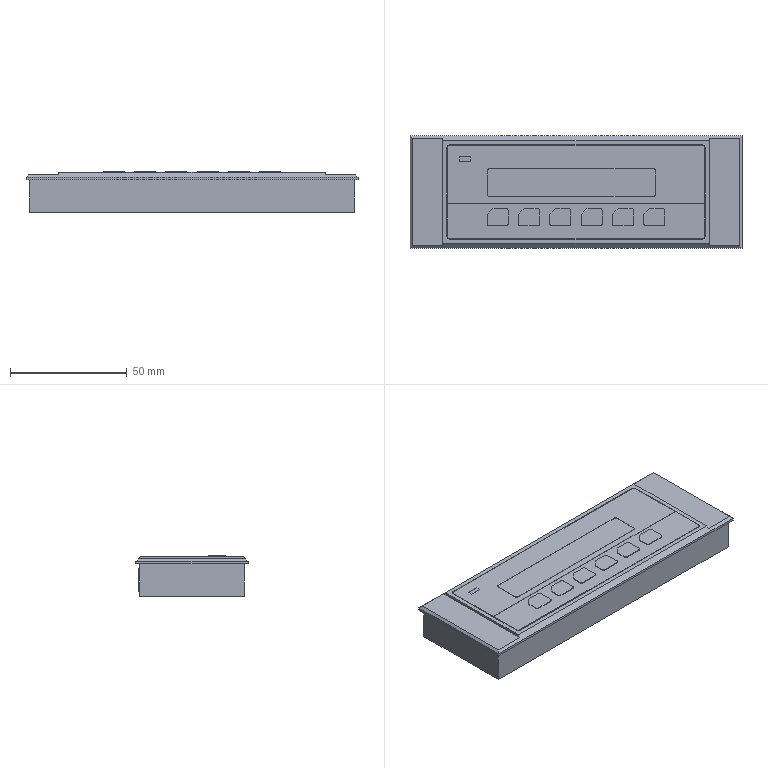Part | STEP file | Vexta Operation Unit OP200A | 1 solid | 117 faces | box 142 x 48 x 17.4 mm | volume 105973 mm3 | plane 87 | cylinder 30 | commonest cylinder face diameters 2 x26 2.4 x4